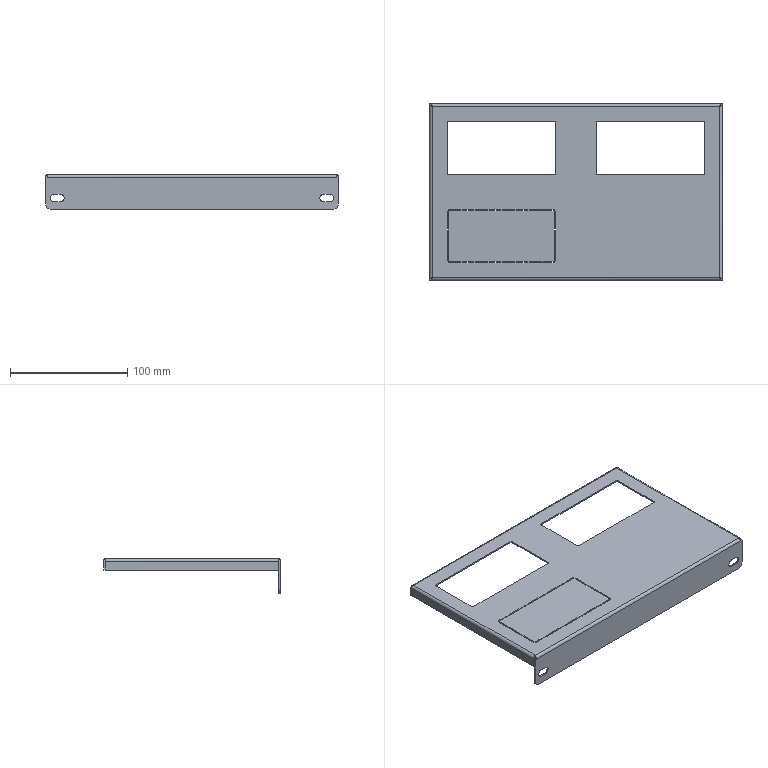Part | SolidWorks | features BaseBody 1 | 1 solid | 184 faces | box 250 x 151 x 30 mm | volume 48403 mm3 | plane 90 | cylinder 86 | spline 8 | commonest cylinder face diameters 1 x72 2.4 x4 4.8 x4 6.5 x4 10 x2